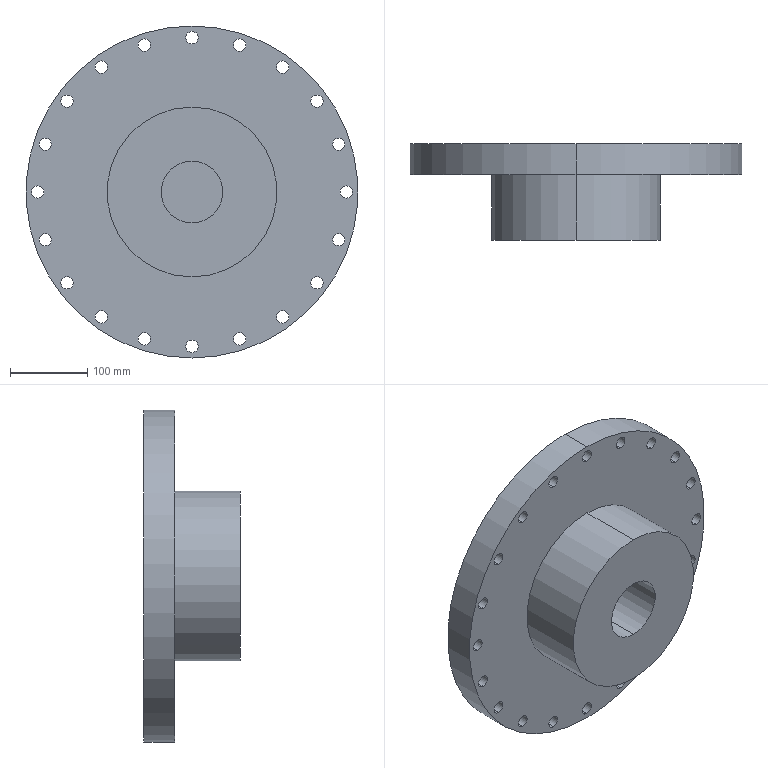Part | SolidWorks | features HoleWzd 2, Extrusion 1, ICE 1 | 1 solid | 50 faces | box 430 x 125 x 430 mm | volume 8451827 mm3 | cylinder 46 | plane 4 | commonest cylinder face diameters 16 x40 80 x2 220 x2 430 x2